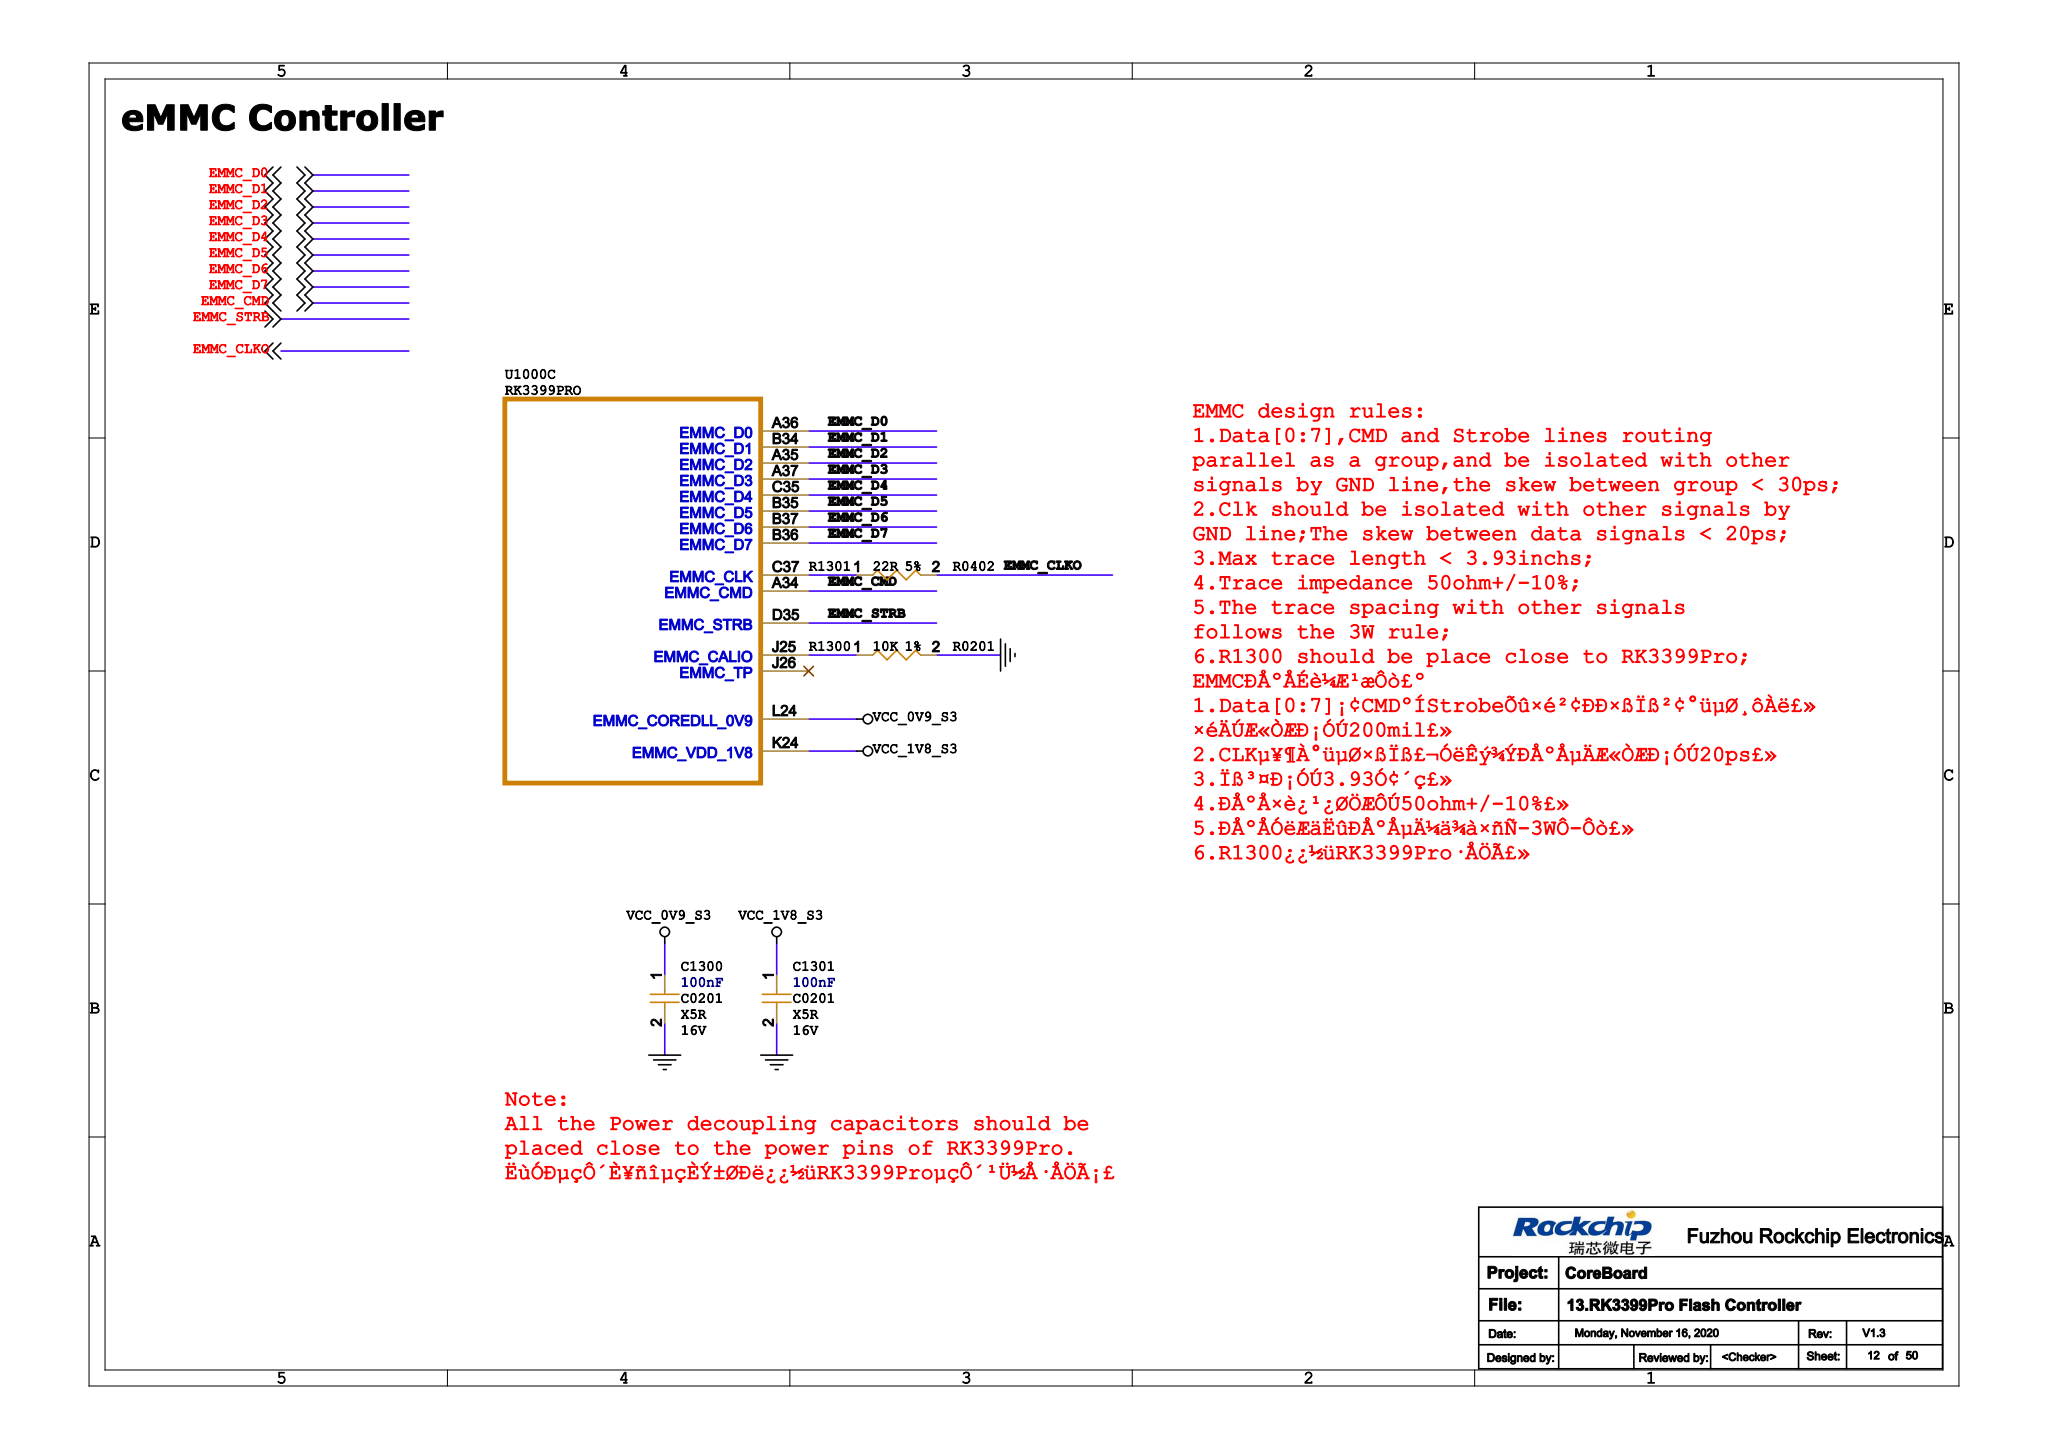Circuit board | Cadence Allegro | 749 parts | 717 nets | one sheet of the schematic
Parts on this sheet (reference | value | footprint):
C1300 | 100nF | C0201
C1301 | 100nF | C0201
U1000 | RK3399PRO | BGA1372_27R00X27R00X2R19
Nets of these parts (net: part-pin ...):
GND: C1300-2 C1301-2
VCC_1V8_S3: C1301-1 U1000-K24
EMMC_CMD: U1000-A34
VCC_0V9_S3: C1300-1 U1000-L24
EMMC_D0: U1000-A36
EMMC_D1: U1000-B34
EMMC_D2: U1000-A35
EMMC_D3: U1000-A37
EMMC_D4: U1000-C35
EMMC_D5: U1000-B35
EMMC_D6: U1000-B37
EMMC_D7: U1000-B36
EMMC_STRB: U1000-D35